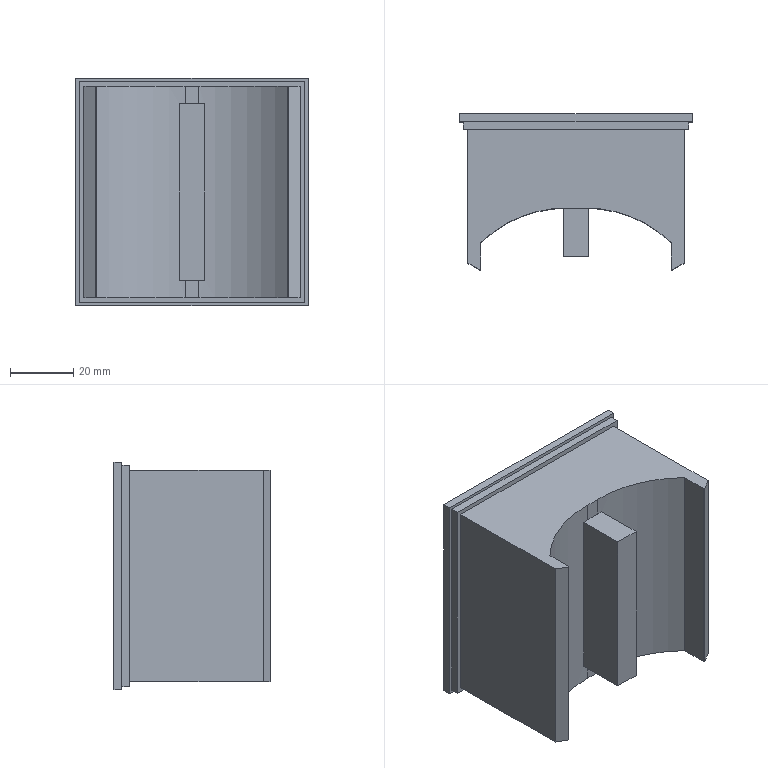Part | SolidWorks | features ICE 4, Extrusion 1 | 1 solid | 36 faces | box 73.144 x 49.228 x 71.78 mm | volume 167014 mm3 | plane 28 | cylinder 8 | commonest cylinder face diameters 3 x4 0.46 x2 77.24 x2
STEP:
#1=CARTESIAN_POINT('',(1.5,16.101,-56.78));
#2=VERTEX_POINT('',#1);
#3=CARTESIAN_POINT('',(-1.5,16.101,-56.78));
#4=VERTEX_POINT('',#3);
#5=CARTESIAN_POINT('',(0.,16.101,-56.78));
#6=DIRECTION('',(0.,0.,-1.));
#7=DIRECTION('',(-1.,0.,0.));
#8=AXIS2_PLACEMENT_3D('',#5,#6,#7);
#9=CIRCLE('',#8,1.5);
#10=EDGE_CURVE('',#2,#4,#9,.T.);
#11=ORIENTED_EDGE('',*,*,#10,.F.);
#12=CARTESIAN_POINT('',(1.5,16.101,-66.78));
#13=VERTEX_POINT('',#12);
#14=CARTESIAN_POINT('',(1.5,16.101,-56.78));
#15=DIRECTION('',(0.,0.,-1.));
#16=VECTOR('',#15,1000.);
#17=LINE('',#14,#16);
#18=EDGE_CURVE('',#2,#13,#17,.T.);
#19=ORIENTED_EDGE('',*,*,#18,.T.);
#20=CARTESIAN_POINT('',(-1.5,16.101,-66.78));
#21=VERTEX_POINT('',#20);
#22=CARTESIAN_POINT('',(0.,16.101,-66.78));
#23=DIRECTION('',(0.,0.,-1.));
#24=DIRECTION('',(-1.,0.,0.));
#25=AXIS2_PLACEMENT_3D('',#22,#23,#24);
#26=CIRCLE('',#25,1.5);
#27=EDGE_CURVE('',#13,#21,#26,.T.);
#28=ORIENTED_EDGE('',*,*,#27,.T.);
#29=CARTESIAN_POINT('',(-1.5,16.101,-56.78));
#30=DIRECTION('',(0.,0.,-1.));
#31=VECTOR('',#30,1000.);
#32=LINE('',#29,#31);
#33=EDGE_CURVE('',#4,#21,#32,.T.);
#34=ORIENTED_EDGE('',*,*,#33,.F.);
#35=EDGE_LOOP('',(#11,#19,#28,#34));
#36=FACE_OUTER_BOUND('',#35,.T.);
#37=CARTESIAN_POINT('',(0.,16.101,-56.78));
#38=DIRECTION('',(0.,0.,-1.));
#39=DIRECTION('',(-1.,0.,0.));
#40=AXIS2_PLACEMENT_3D('',#37,#38,#39);
#41=CYLINDRICAL_SURFACE('',#40,1.5);
#42=ADVANCED_FACE('',(#36),#41,.F.);
#43=CARTESIAN_POINT('',(1.5,6.101,-56.78));
#44=VERTEX_POINT('',#43);
#45=CARTESIAN_POINT('',(-1.5,6.101,-56.78));
#46=VERTEX_POINT('',#45);
#47=CARTESIAN_POINT('',(0.,6.101,-56.78));
#48=DIRECTION('',(0.,0.,-1.));
#49=DIRECTION('',(-1.,0.,0.));
#50=AXIS2_PLACEMENT_3D('',#47,#48,#49);
#51=CIRCLE('',#50,1.5);
#52=EDGE_CURVE('',#44,#46,#51,.T.);
#53=ORIENTED_EDGE('',*,*,#52,.F.);
#54=CARTESIAN_POINT('',(1.5,6.101,-66.78));
#55=VERTEX_POINT('',#54);
#56=CARTESIAN_POINT('',(1.5,6.101,-56.78));
#57=DIRECTION('',(0.,0.,-1.));
#58=VECTOR('',#57,1000.);
#59=LINE('',#56,#58);
#60=EDGE_CURVE('',#44,#55,#59,.T.);
#61=ORIENTED_EDGE('',*,*,#60,.T.);
#62=CARTESIAN_POINT('',(-1.5,6.101,-66.78));
#63=VERTEX_POINT('',#62);
#64=CARTESIAN_POINT('',(0.,6.101,-66.78));
#65=DIRECTION('',(0.,0.,-1.));
#66=DIRECTION('',(-1.,0.,0.));
#67=AXIS2_PLACEMENT_3D('',#64,#65,#66);
#68=CIRCLE('',#67,1.5);
#69=EDGE_CURVE('',#55,#63,#68,.T.);
#70=ORIENTED_EDGE('',*,*,#69,.T.);
#71=CARTESIAN_POINT('',(-1.5,6.101,-56.78));
#72=DIRECTION('',(0.,0.,-1.));
#73=VECTOR('',#72,1000.);
#74=LINE('',#71,#73);
#75=EDGE_CURVE('',#46,#63,#74,.T.);
#76=ORIENTED_EDGE('',*,*,#75,.F.);
#77=EDGE_LOOP('',(#53,#61,#70,#76));
#78=FACE_OUTER_BOUND('',#77,.T.);
#79=CARTESIAN_POINT('',(0.,6.101,-56.78));
#80=DIRECTION('',(0.,0.,-1.));
#81=DIRECTION('',(-1.,0.,0.));
#82=AXIS2_PLACEMENT_3D('',#79,#80,#81);
#83=CYLINDRICAL_SURFACE('',#82,1.5);
#84=ADVANCED_FACE('',(#78),#83,.F.);
#85=CARTESIAN_POINT('',(-2.201,0.77,-61.17));
#86=VERTEX_POINT('',#85);
#87=CARTESIAN_POINT('',(2.201,0.77,-61.17));
#88=VERTEX_POINT('',#87);
#89=CARTESIAN_POINT('',(0.,0.77,-61.17));
#90=DIRECTION('',(1.,0.,0.));
#91=VECTOR('',#90,1000.);
#92=LINE('',#89,#91);
#93=EDGE_CURVE('',#86,#88,#92,.T.);
#94=ORIENTED_EDGE('',*,*,#93,.F.);
#95=CARTESIAN_POINT('',(-2.201,0.77,-66.78));
#96=VERTEX_POINT('',#95);
#97=CARTESIAN_POINT('',(-2.201,0.77,-66.78));
#98=DIRECTION('',(0.,0.,1.));
#99=VECTOR('',#98,1000.);
#100=LINE('',#97,#99);
#101=EDGE_CURVE('',#96,#86,#100,.T.);
#102=ORIENTED_EDGE('',*,*,#101,.F.);
#103=CARTESIAN_POINT('',(2.201,0.77,-66.78));
#104=VERTEX_POINT('',#103);
#105=CARTESIAN_POINT('',(0.,0.77,-66.78));
#106=DIRECTION('',(1.,0.,0.));
#107=VECTOR('',#106,1000.);
#108=LINE('',#105,#107);
#109=EDGE_CURVE('',#96,#104,#108,.T.);
#110=ORIENTED_EDGE('',*,*,#109,.T.);
#111=CARTESIAN_POINT('',(2.201,0.77,-66.78));
#112=DIRECTION('',(0.,0.,1.));
#113=VECTOR('',#112,1000.);
#114=LINE('',#111,#113);
#115=EDGE_CURVE('',#104,#88,#114,.T.);
#116=ORIENTED_EDGE('',*,*,#115,.T.);
#117=EDGE_LOOP('',(#94,#102,#110,#116));
#118=FACE_OUTER_BOUND('',#117,.T.);
#119=CARTESIAN_POINT('',(0.,0.77,-66.78));
#120=DIRECTION('',(0.,-1.,0.));
#121=DIRECTION('',(1.,0.,0.));
#122=AXIS2_PLACEMENT_3D('',#119,#120,#121);
#123=PLANE('',#122);
#124=ADVANCED_FACE('',(#118),#123,.T.);
#125=CARTESIAN_POINT('',(-34.072,25.498,0.));
#126=VERTEX_POINT('',#125);
#127=CARTESIAN_POINT('',(-34.072,-16.562,0.));
#128=VERTEX_POINT('',#127);
#129=CARTESIAN_POINT('',(-34.072,-16.562,0.));
#130=DIRECTION('',(0.,-1.,0.));
#131=VECTOR('',#130,1000.);
#132=LINE('',#129,#131);
#133=EDGE_CURVE('',#126,#128,#132,.T.);
#134=ORIENTED_EDGE('',*,*,#133,.F.);
#135=CARTESIAN_POINT('',(-34.072,25.498,-66.78));
#136=VERTEX_POINT('',#135);
#137=CARTESIAN_POINT('',(-34.072,25.498,-66.78));
#138=DIRECTION('',(0.,0.,1.));
#139=VECTOR('',#138,1000.);
#140=LINE('',#137,#139);
#141=EDGE_CURVE('',#136,#126,#140,.T.);
#142=ORIENTED_EDGE('',*,*,#141,.F.);
#143=CARTESIAN_POINT('',(-34.072,-16.562,-66.78));
#144=VERTEX_POINT('',#143);
#145=CARTESIAN_POINT('',(-34.072,-16.562,-66.78));
#146=DIRECTION('',(0.,-1.,0.));
#147=VECTOR('',#146,1000.);
#148=LINE('',#145,#147);
#149=EDGE_CURVE('',#136,#144,#148,.T.);
#150=ORIENTED_EDGE('',*,*,#149,.T.);
#151=CARTESIAN_POINT('',(-34.072,-16.562,-66.78));
#152=DIRECTION('',(0.,0.,1.));
#153=VECTOR('',#152,1000.);
#154=LINE('',#151,#153);
#155=EDGE_CURVE('',#144,#128,#154,.T.);
#156=ORIENTED_EDGE('',*,*,#155,.T.);
#157=EDGE_LOOP('',(#134,#142,#150,#156));
#158=FACE_OUTER_BOUND('',#157,.T.);
#159=CARTESIAN_POINT('',(-34.072,-16.562,-66.78));
#160=DIRECTION('',(-1.,0.,0.));
#161=DIRECTION('',(0.,0.,1.));
#162=AXIS2_PLACEMENT_3D('',#159,#160,#161);
#163=PLANE('',#162);
#164=ADVANCED_FACE('',(#158),#163,.T.);
#165=CARTESIAN_POINT('',(34.072,-16.562,0.));
#166=VERTEX_POINT('',#165);
#167=CARTESIAN_POINT('',(34.072,25.498,0.));
#168=VERTEX_POINT('',#167);
#169=CARTESIAN_POINT('',(34.072,-16.562,0.));
#170=DIRECTION('',(0.,1.,0.));
#171=VECTOR('',#170,1000.);
#172=LINE('',#169,#171);
#173=EDGE_CURVE('',#166,#168,#172,.T.);
#174=ORIENTED_EDGE('',*,*,#173,.F.);
#175=CARTESIAN_POINT('',(34.072,-16.562,-66.78));
#176=VERTEX_POINT('',#175);
#177=CARTESIAN_POINT('',(34.072,-16.562,-66.78));
#178=DIRECTION('',(0.,0.,1.));
#179=VECTOR('',#178,1000.);
#180=LINE('',#177,#179);
#181=EDGE_CURVE('',#176,#166,#180,.T.);
#182=ORIENTED_EDGE('',*,*,#181,.F.);
#183=CARTESIAN_POINT('',(34.072,25.498,-66.78));
#184=VERTEX_POINT('',#183);
#185=CARTESIAN_POINT('',(34.072,-16.562,-66.78));
#186=DIRECTION('',(0.,1.,0.));
#187=VECTOR('',#186,1000.);
#188=LINE('',#185,#187);
#189=EDGE_CURVE('',#176,#184,#188,.T.);
#190=ORIENTED_EDGE('',*,*,#189,.T.);
#191=CARTESIAN_POINT('',(34.072,25.498,-66.78));
#192=DIRECTION('',(0.,0.,1.));
#193=VECTOR('',#192,1000.);
#194=LINE('',#191,#193);
#195=EDGE_CURVE('',#184,#168,#194,.T.);
#196=ORIENTED_EDGE('',*,*,#195,.T.);
#197=EDGE_LOOP('',(#174,#182,#190,#196));
#198=FACE_OUTER_BOUND('',#197,.T.);
#199=CARTESIAN_POINT('',(34.072,-16.562,-66.78));
#200=DIRECTION('',(1.,0.,0.));
#201=DIRECTION('',(0.,1.,0.));
#202=AXIS2_PLACEMENT_3D('',#199,#200,#201);
#203=PLANE('',#202);
#204=ADVANCED_FACE('',(#198),#203,.T.);
#205=CARTESIAN_POINT('',(30.37,-18.699,0.));
#206=VERTEX_POINT('',#205);
#207=CARTESIAN_POINT('',(30.37,-18.699,0.));
#208=DIRECTION('',(0.866,0.5,0.));
#209=VECTOR('',#208,1000.);
#210=LINE('',#207,#209);
#211=EDGE_CURVE('',#206,#166,#210,.T.);
#212=ORIENTED_EDGE('',*,*,#211,.F.);
#213=CARTESIAN_POINT('',(30.37,-18.699,-66.78));
#214=VERTEX_POINT('',#213);
#215=CARTESIAN_POINT('',(30.37,-18.699,-66.78));
#216=DIRECTION('',(0.,0.,1.));
#217=VECTOR('',#216,1000.);
#218=LINE('',#215,#217);
#219=EDGE_CURVE('',#214,#206,#218,.T.);
#220=ORIENTED_EDGE('',*,*,#219,.F.);
#221=CARTESIAN_POINT('',(30.37,-18.699,-66.78));
#222=DIRECTION('',(0.866,0.5,0.));
#223=VECTOR('',#222,1000.);
#224=LINE('',#221,#223);
#225=EDGE_CURVE('',#214,#176,#224,.T.);
#226=ORIENTED_EDGE('',*,*,#225,.T.);
#227=ORIENTED_EDGE('',*,*,#181,.T.);
#228=EDGE_LOOP('',(#212,#220,#226,#227));
#229=FACE_OUTER_BOUND('',#228,.T.);
#230=CARTESIAN_POINT('',(30.37,-18.699,-66.78));
#231=DIRECTION('',(0.5,-0.866,0.));
#232=DIRECTION('',(0.866,0.5,0.));
#233=AXIS2_PLACEMENT_3D('',#230,#231,#232);
#234=PLANE('',#233);
#235=ADVANCED_FACE('',(#229),#234,.T.);
#236=CARTESIAN_POINT('',(30.025,-18.5,0.));
#237=VERTEX_POINT('',#236);
#238=CARTESIAN_POINT('',(30.255,-18.5,0.));
#239=DIRECTION('',(0.,0.,1.));
#240=DIRECTION('',(-1.,0.,0.));
#241=AXIS2_PLACEMENT_3D('',#238,#239,#240);
#242=CIRCLE('',#241,0.23);
#243=EDGE_CURVE('',#237,#206,#242,.T.);
#244=ORIENTED_EDGE('',*,*,#243,.F.);
#245=CARTESIAN_POINT('',(30.025,-18.5,-66.78));
#246=VERTEX_POINT('',#245);
#247=CARTESIAN_POINT('',(30.025,-18.5,-66.78));
#248=DIRECTION('',(0.,0.,1.));
#249=VECTOR('',#248,1000.);
#250=LINE('',#247,#249);
#251=EDGE_CURVE('',#246,#237,#250,.T.);
#252=ORIENTED_EDGE('',*,*,#251,.F.);
#253=CARTESIAN_POINT('',(30.255,-18.5,-66.78));
#254=DIRECTION('',(0.,0.,1.));
#255=DIRECTION('',(-1.,0.,0.));
#256=AXIS2_PLACEMENT_3D('',#253,#254,#255);
#257=CIRCLE('',#256,0.23);
#258=EDGE_CURVE('',#246,#214,#257,.T.);
#259=ORIENTED_EDGE('',*,*,#258,.T.);
#260=ORIENTED_EDGE('',*,*,#219,.T.);
#261=EDGE_LOOP('',(#244,#252,#259,#260));
#262=FACE_OUTER_BOUND('',#261,.T.);
#263=CARTESIAN_POINT('',(30.255,-18.5,-66.78));
#264=DIRECTION('',(0.,0.,1.));
#265=DIRECTION('',(1.,0.,0.));
#266=AXIS2_PLACEMENT_3D('',#263,#264,#265);
#267=CYLINDRICAL_SURFACE('',#266,0.23);
#268=ADVANCED_FACE('',(#262),#267,.T.);
#269=CARTESIAN_POINT('',(30.025,-10.173,0.));
#270=VERTEX_POINT('',#269);
#271=CARTESIAN_POINT('',(30.025,-10.173,0.));
#272=DIRECTION('',(0.,-1.,0.));
#273=VECTOR('',#272,1000.);
#274=LINE('',#271,#273);
#275=EDGE_CURVE('',#270,#237,#274,.T.);
#276=ORIENTED_EDGE('',*,*,#275,.F.);
#277=CARTESIAN_POINT('',(30.025,-10.173,-66.78));
#278=VERTEX_POINT('',#277);
#279=CARTESIAN_POINT('',(30.025,-10.173,-66.78));
#280=DIRECTION('',(0.,0.,1.));
#281=VECTOR('',#280,1000.);
#282=LINE('',#279,#281);
#283=EDGE_CURVE('',#278,#270,#282,.T.);
#284=ORIENTED_EDGE('',*,*,#283,.F.);
#285=CARTESIAN_POINT('',(30.025,-10.173,-66.78));
#286=DIRECTION('',(0.,-1.,0.));
#287=VECTOR('',#286,1000.);
#288=LINE('',#285,#287);
#289=EDGE_CURVE('',#278,#246,#288,.T.);
#290=ORIENTED_EDGE('',*,*,#289,.T.);
#291=ORIENTED_EDGE('',*,*,#251,.T.);
#292=EDGE_LOOP('',(#276,#284,#290,#291));
#293=FACE_OUTER_BOUND('',#292,.T.);
#294=CARTESIAN_POINT('',(30.025,-10.173,-66.78));
#295=DIRECTION('',(-1.,0.,0.));
#296=DIRECTION('',(0.,-1.,0.));
#297=AXIS2_PLACEMENT_3D('',#294,#295,#296);
#298=PLANE('',#297);
#299=ADVANCED_FACE('',(#293),#298,.T.);
#300=CARTESIAN_POINT('',(4.03,0.7683,-61.17));
#301=VERTEX_POINT('',#300);
#302=CARTESIAN_POINT('',(3.08,-37.84,-61.17));
#303=DIRECTION('',(0.,0.,-1.));
#304=DIRECTION('',(-1.,0.,0.));
#305=AXIS2_PLACEMENT_3D('',#302,#303,#304);
#306=CIRCLE('',#305,38.62);
#307=EDGE_CURVE('',#88,#301,#306,.T.);
#308=ORIENTED_EDGE('',*,*,#307,.F.);
#309=ORIENTED_EDGE('',*,*,#115,.F.);
#310=CARTESIAN_POINT('',(3.08,-37.84,-66.78));
#311=DIRECTION('',(0.,0.,-1.));
#312=DIRECTION('',(-1.,0.,0.));
#313=AXIS2_PLACEMENT_3D('',#310,#311,#312);
#314=CIRCLE('',#313,38.62);
#315=EDGE_CURVE('',#104,#278,#314,.T.);
#316=ORIENTED_EDGE('',*,*,#315,.T.);
#317=ORIENTED_EDGE('',*,*,#283,.T.);
#318=CARTESIAN_POINT('',(2.201,0.77,0.));
#319=VERTEX_POINT('',#318);
#320=CARTESIAN_POINT('',(3.08,-37.84,0.));
#321=DIRECTION('',(0.,0.,-1.));
#322=DIRECTION('',(-1.,0.,0.));
#323=AXIS2_PLACEMENT_3D('',#320,#321,#322);
#324=CIRCLE('',#323,38.62);
#325=EDGE_CURVE('',#319,#270,#324,.T.);
#326=ORIENTED_EDGE('',*,*,#325,.F.);
#327=CARTESIAN_POINT('',(2.201,0.77,-5.61));
#328=VERTEX_POINT('',#327);
#329=CARTESIAN_POINT('',(2.201,0.77,-66.78));
#330=DIRECTION('',(0.,0.,1.));
#331=VECTOR('',#330,1000.);
#332=LINE('',#329,#331);
#333=EDGE_CURVE('',#328,#319,#332,.T.);
#334=ORIENTED_EDGE('',*,*,#333,.F.);
#335=CARTESIAN_POINT('',(4.03,0.7683,-5.61));
#336=VERTEX_POINT('',#335);
#337=CARTESIAN_POINT('',(3.08,-37.84,-5.61));
#338=DIRECTION('',(0.,0.,1.));
#339=DIRECTION('',(1.,0.,0.));
#340=AXIS2_PLACEMENT_3D('',#337,#338,#339);
#341=CIRCLE('',#340,38.62);
#342=EDGE_CURVE('',#336,#328,#341,.T.);
#343=ORIENTED_EDGE('',*,*,#342,.F.);
#344=CARTESIAN_POINT('',(4.03,0.7683,-66.78));
#345=DIRECTION('',(0.,0.,1.));
#346=VECTOR('',#345,1000.);
#347=LINE('',#344,#346);
#348=EDGE_CURVE('',#301,#336,#347,.T.);
#349=ORIENTED_EDGE('',*,*,#348,.F.);
#350=EDGE_LOOP('',(#308,#309,#316,#317,#326,#334,#343,#349));
#351=FACE_OUTER_BOUND('',#350,.T.);
#352=CARTESIAN_POINT('',(3.08,-37.84,-66.78));
#353=DIRECTION('',(0.,0.,1.));
#354=DIRECTION('',(1.,0.,0.));
#355=AXIS2_PLACEMENT_3D('',#352,#353,#354);
#356=CYLINDRICAL_SURFACE('',#355,38.62);
#357=ADVANCED_FACE('',(#351),#356,.F.);
#358=CARTESIAN_POINT('',(-2.201,0.77,-5.61));
#359=VERTEX_POINT('',#358);
#360=CARTESIAN_POINT('',(0.,0.77,-5.61));
#361=DIRECTION('',(-1.,0.,0.));
#362=VECTOR('',#361,1000.);
#363=LINE('',#360,#362);
#364=EDGE_CURVE('',#328,#359,#363,.T.);
#365=ORIENTED_EDGE('',*,*,#364,.F.);
#366=ORIENTED_EDGE('',*,*,#333,.T.);
#367=CARTESIAN_POINT('',(-2.201,0.77,0.));
#368=VERTEX_POINT('',#367);
#369=CARTESIAN_POINT('',(0.,0.77,0.));
#370=DIRECTION('',(1.,0.,0.));
#371=VECTOR('',#370,1000.);
#372=LINE('',#369,#371);
#373=EDGE_CURVE('',#368,#319,#372,.T.);
#374=ORIENTED_EDGE('',*,*,#373,.F.);
#375=CARTESIAN_POINT('',(-2.201,0.77,-66.78));
#376=DIRECTION('',(0.,0.,1.));
#377=VECTOR('',#376,1000.);
#378=LINE('',#375,#377);
#379=EDGE_CURVE('',#359,#368,#378,.T.);
#380=ORIENTED_EDGE('',*,*,#379,.F.);
#381=EDGE_LOOP('',(#365,#366,#374,#380));
#382=FACE_OUTER_BOUND('',#381,.T.);
#383=CARTESIAN_POINT('',(0.,0.77,-66.78));
#384=DIRECTION('',(0.,-1.,0.));
#385=DIRECTION('',(1.,0.,0.));
#386=AXIS2_PLACEMENT_3D('',#383,#384,#385);
#387=PLANE('',#386);
#388=ADVANCED_FACE('',(#382),#387,.T.);
#389=CARTESIAN_POINT('',(-4.03,0.7683,-61.17));
#390=VERTEX_POINT('',#389);
#391=CARTESIAN_POINT('',(-3.08,-37.84,-61.17));
#392=DIRECTION('',(0.,0.,-1.));
#393=DIRECTION('',(-1.,0.,0.));
#394=AXIS2_PLACEMENT_3D('',#391,#392,#393);
#395=CIRCLE('',#394,38.62);
#396=EDGE_CURVE('',#390,#86,#395,.T.);
#397=ORIENTED_EDGE('',*,*,#396,.F.);
#398=CARTESIAN_POINT('',(-4.03,0.7683,-5.61));
#399=VERTEX_POINT('',#398);
#400=CARTESIAN_POINT('',(-4.03,0.7683,-66.78));
#401=DIRECTION('',(0.,0.,-1.));
#402=VECTOR('',#401,1000.);
#403=LINE('',#400,#402);
#404=EDGE_CURVE('',#399,#390,#403,.T.);
#405=ORIENTED_EDGE('',*,*,#404,.F.);
#406=CARTESIAN_POINT('',(-3.08,-37.84,-5.61));
#407=DIRECTION('',(0.,0.,1.));
#408=DIRECTION('',(1.,0.,0.));
#409=AXIS2_PLACEMENT_3D('',#406,#407,#408);
#410=CIRCLE('',#409,38.62);
#411=EDGE_CURVE('',#359,#399,#410,.T.);
#412=ORIENTED_EDGE('',*,*,#411,.F.);
#413=ORIENTED_EDGE('',*,*,#379,.T.);
#414=CARTESIAN_POINT('',(-30.025,-10.173,0.));
#415=VERTEX_POINT('',#414);
#416=CARTESIAN_POINT('',(-3.08,-37.84,0.));
#417=DIRECTION('',(0.,0.,-1.));
#418=DIRECTION('',(1.,0.,0.));
#419=AXIS2_PLACEMENT_3D('',#416,#417,#418);
#420=CIRCLE('',#419,38.62);
#421=EDGE_CURVE('',#415,#368,#420,.T.);
#422=ORIENTED_EDGE('',*,*,#421,.F.);
#423=CARTESIAN_POINT('',(-30.025,-10.173,-66.78));
#424=VERTEX_POINT('',#423);
#425=CARTESIAN_POINT('',(-30.025,-10.173,-66.78));
#426=DIRECTION('',(0.,0.,1.));
#427=VECTOR('',#426,1000.);
#428=LINE('',#425,#427);
#429=EDGE_CURVE('',#424,#415,#428,.T.);
#430=ORIENTED_EDGE('',*,*,#429,.F.);
#431=CARTESIAN_POINT('',(-3.08,-37.84,-66.78));
#432=DIRECTION('',(0.,0.,-1.));
#433=DIRECTION('',(1.,0.,0.));
#434=AXIS2_PLACEMENT_3D('',#431,#432,#433);
#435=CIRCLE('',#434,38.62);
#436=EDGE_CURVE('',#424,#96,#435,.T.);
#437=ORIENTED_EDGE('',*,*,#436,.T.);
#438=ORIENTED_EDGE('',*,*,#101,.T.);
#439=EDGE_LOOP('',(#397,#405,#412,#413,#422,#430,#437,#438));
#440=FACE_OUTER_BOUND('',#439,.T.);
#441=CARTESIAN_POINT('',(-3.08,-37.84,-66.78));
#442=DIRECTION('',(0.,0.,1.));
#443=DIRECTION('',(1.,0.,0.));
#444=AXIS2_PLACEMENT_3D('',#441,#442,#443);
#445=CYLINDRICAL_SURFACE('',#444,38.62);
#446=ADVANCED_FACE('',(#440),#445,.F.);
#447=CARTESIAN_POINT('',(-30.025,-18.5,0.));
#448=VERTEX_POINT('',#447);
#449=CARTESIAN_POINT('',(-30.025,-10.173,0.));
#450=DIRECTION('',(0.,1.,0.));
#451=VECTOR('',#450,1000.);
#452=LINE('',#449,#451);
#453=EDGE_CURVE('',#448,#415,#452,.T.);
#454=ORIENTED_EDGE('',*,*,#453,.F.);
#455=CARTESIAN_POINT('',(-30.025,-18.5,-66.78));
#456=VERTEX_POINT('',#455);
#457=CARTESIAN_POINT('',(-30.025,-18.5,-66.78));
#458=DIRECTION('',(0.,0.,1.));
#459=VECTOR('',#458,1000.);
#460=LINE('',#457,#459);
#461=EDGE_CURVE('',#456,#448,#460,.T.);
#462=ORIENTED_EDGE('',*,*,#461,.F.);
#463=CARTESIAN_POINT('',(-30.025,-10.173,-66.78));
#464=DIRECTION('',(0.,1.,0.));
#465=VECTOR('',#464,1000.);
#466=LINE('',#463,#465);
#467=EDGE_CURVE('',#456,#424,#466,.T.);
#468=ORIENTED_EDGE('',*,*,#467,.T.);
#469=ORIENTED_EDGE('',*,*,#429,.T.);
#470=EDGE_LOOP('',(#454,#462,#468,#469));
#471=FACE_OUTER_BOUND('',#470,.T.);
#472=CARTESIAN_POINT('',(-30.025,-10.173,-66.78));
#473=DIRECTION('',(1.,0.,0.));
#474=DIRECTION('',(0.,1.,0.));
#475=AXIS2_PLACEMENT_3D('',#472,#473,#474);
#476=PLANE('',#475);
#477=ADVANCED_FACE('',(#471),#476,.T.);
#478=CARTESIAN_POINT('',(-30.37,-18.699,0.));
#479=VERTEX_POINT('',#478);
#480=CARTESIAN_POINT('',(-30.255,-18.5,0.));
#481=DIRECTION('',(0.,0.,1.));
#482=DIRECTION('',(1.,0.,0.));
#483=AXIS2_PLACEMENT_3D('',#480,#481,#482);
#484=CIRCLE('',#483,0.23);
#485=EDGE_CURVE('',#479,#448,#484,.T.);
#486=ORIENTED_EDGE('',*,*,#485,.F.);
#487=CARTESIAN_POINT('',(-30.37,-18.699,-66.78));
#488=VERTEX_POINT('',#487);
#489=CARTESIAN_POINT('',(-30.37,-18.699,-66.78));
#490=DIRECTION('',(0.,0.,1.));
#491=VECTOR('',#490,1000.);
#492=LINE('',#489,#491);
#493=EDGE_CURVE('',#488,#479,#492,.T.);
#494=ORIENTED_EDGE('',*,*,#493,.F.);
#495=CARTESIAN_POINT('',(-30.255,-18.5,-66.78));
#496=DIRECTION('',(0.,0.,1.));
#497=DIRECTION('',(1.,0.,0.));
#498=AXIS2_PLACEMENT_3D('',#495,#496,#497);
#499=CIRCLE('',#498,0.23);
#500=EDGE_CURVE('',#488,#456,#499,.T.);
#501=ORIENTED_EDGE('',*,*,#500,.T.);
#502=ORIENTED_EDGE('',*,*,#461,.T.);
#503=EDGE_LOOP('',(#486,#494,#501,#502));
#504=FACE_OUTER_BOUND('',#503,.T.);
#505=CARTESIAN_POINT('',(-30.255,-18.5,-66.78));
#506=DIRECTION('',(0.,0.,1.));
#507=DIRECTION('',(1.,0.,0.));
#508=AXIS2_PLACEMENT_3D('',#505,#506,#507);
#509=CYLINDRICAL_SURFACE('',#508,0.23);
#510=ADVANCED_FACE('',(#504),#509,.T.);
#511=CARTESIAN_POINT('',(-30.37,-18.699,0.));
#512=DIRECTION('',(0.866,-0.5,0.));
#513=VECTOR('',#512,1000.);
#514=LINE('',#511,#513);
#515=EDGE_CURVE('',#128,#479,#514,.T.);
#516=ORIENTED_EDGE('',*,*,#515,.F.);
#517=ORIENTED_EDGE('',*,*,#155,.F.);
#518=CARTESIAN_POINT('',(-30.37,-18.699,-66.78));
#519=DIRECTION('',(0.866,-0.5,0.));
#520=VECTOR('',#519,1000.);
#521=LINE('',#518,#520);
#522=EDGE_CURVE('',#144,#488,#521,.T.);
#523=ORIENTED_EDGE('',*,*,#522,.T.);
#524=ORIENTED_EDGE('',*,*,#493,.T.);
#525=EDGE_LOOP('',(#516,#517,#523,#524));
#526=FACE_OUTER_BOUND('',#525,.T.);
#527=CARTESIAN_POINT('',(-30.37,-18.699,-66.78));
#528=DIRECTION('',(-0.5,-0.866,0.));
#529=DIRECTION('',(0.866,-0.5,0.));
#530=AXIS2_PLACEMENT_3D('',#527,#528,#529);
#531=PLANE('',#530);
#532=ADVANCED_FACE('',(#526),#531,.T.);
#533=CARTESIAN_POINT('',(0.,16.101,-66.78));
#534=DIRECTION('',(0.,0.,-1.));
#535=DIRECTION('',(-1.,0.,0.));
#536=AXIS2_PLACEMENT_3D('',#533,#534,#535);
#537=CIRCLE('',#536,1.5);
#538=EDGE_CURVE('',#21,#13,#537,.T.);
#539=ORIENTED_EDGE('',*,*,#538,.F.);
#540=ORIENTED_EDGE('',*,*,#27,.F.);
#541=EDGE_LOOP('',(#539,#540));
#542=FACE_BOUND('',#541,.T.);
#543=CARTESIAN_POINT('',(0.,6.101,-66.78));
#544=DIRECTION('',(0.,0.,-1.));
#545=DIRECTION('',(-1.,0.,0.));
#546=AXIS2_PLACEMENT_3D('',#543,#544,#545);
#547=CIRCLE('',#546,1.5);
#548=EDGE_CURVE('',#63,#55,#547,.T.);
#549=ORIENTED_EDGE('',*,*,#548,.F.);
#550=ORIENTED_EDGE('',*,*,#69,.F.);
#551=EDGE_LOOP('',(#549,#550));
#552=FACE_BOUND('',#551,.T.);
#553=ORIENTED_EDGE('',*,*,#149,.F.);
#554=CARTESIAN_POINT('',(-34.072,25.498,-66.78));
#555=DIRECTION('',(-1.,0.,0.));
#556=VECTOR('',#555,1000.);
#557=LINE('',#554,#556);
#558=EDGE_CURVE('',#184,#136,#557,.T.);
#559=ORIENTED_EDGE('',*,*,#558,.F.);
#560=ORIENTED_EDGE('',*,*,#189,.F.);
#561=ORIENTED_EDGE('',*,*,#225,.F.);
#562=ORIENTED_EDGE('',*,*,#258,.F.);
#563=ORIENTED_EDGE('',*,*,#289,.F.);
#564=ORIENTED_EDGE('',*,*,#315,.F.);
#565=ORIENTED_EDGE('',*,*,#109,.F.);
#566=ORIENTED_EDGE('',*,*,#436,.F.);
#567=ORIENTED_EDGE('',*,*,#467,.F.);
#568=ORIENTED_EDGE('',*,*,#500,.F.);
#569=ORIENTED_EDGE('',*,*,#522,.F.);
#570=EDGE_LOOP('',(#553,#559,#560,#561,#562,#563,#564,#565,#566,#567,#568,#569));
#571=FACE_OUTER_BOUND('',#570,.T.);
#572=CARTESIAN_POINT('',(30.255,-18.5,-66.78));
#573=DIRECTION('',(0.,0.,-1.));
#574=DIRECTION('',(-1.,0.,0.));
#575=AXIS2_PLACEMENT_3D('',#572,#573,#574);
#576=PLANE('',#575);
#577=ADVANCED_FACE('',(#542,#552,#571),#576,.T.);
#578=ORIENTED_EDGE('',*,*,#133,.T.);
#579=ORIENTED_EDGE('',*,*,#515,.T.);
#580=ORIENTED_EDGE('',*,*,#485,.T.);
#581=ORIENTED_EDGE('',*,*,#453,.T.);
#582=ORIENTED_EDGE('',*,*,#421,.T.);
#583=ORIENTED_EDGE('',*,*,#373,.T.);
#584=ORIENTED_EDGE('',*,*,#325,.T.);
#585=ORIENTED_EDGE('',*,*,#275,.T.);
#586=ORIENTED_EDGE('',*,*,#243,.T.);
#587=ORIENTED_EDGE('',*,*,#211,.T.);
#588=ORIENTED_EDGE('',*,*,#173,.T.);
#589=CARTESIAN_POINT('',(-34.072,25.498,0.));
#590=DIRECTION('',(-1.,0.,0.));
#591=VECTOR('',#590,1000.);
#592=LINE('',#589,#591);
#593=EDGE_CURVE('',#168,#126,#592,.T.);
#594=ORIENTED_EDGE('',*,*,#593,.T.);
#595=EDGE_LOOP('',(#578,#579,#580,#581,#582,#583,#584,#585,#586,#587,#588,#594));
#596=FACE_OUTER_BOUND('',#595,.T.);
#597=CARTESIAN_POINT('',(30.255,-18.5,0.));
#598=DIRECTION('',(0.,0.,-1.));
#599=DIRECTION('',(-1.,0.,0.));
#600=AXIS2_PLACEMENT_3D('',#597,#598,#599);
#601=PLANE('',#600);
#602=ADVANCED_FACE('',(#596),#601,.F.);
#603=ORIENTED_EDGE('',*,*,#93,.T.);
#604=ORIENTED_EDGE('',*,*,#307,.T.);
#605=CARTESIAN_POINT('',(4.03,-14.502,-61.17));
#606=VERTEX_POINT('',#605);
#607=CARTESIAN_POINT('',(4.03,-14.502,-61.17));
#608=DIRECTION('',(0.,1.,0.));
#609=VECTOR('',#608,1000.);
#610=LINE('',#607,#609);
#611=EDGE_CURVE('',#606,#301,#610,.T.);
#612=ORIENTED_EDGE('',*,*,#611,.F.);
#613=CARTESIAN_POINT('',(-4.03,-14.502,-61.17));
#614=VERTEX_POINT('',#613);
#615=CARTESIAN_POINT('',(4.03,-14.502,-61.17));
#616=DIRECTION('',(-1.,0.,0.));
#617=VECTOR('',#616,1000.);
#618=LINE('',#615,#617);
#619=EDGE_CURVE('',#606,#614,#618,.T.);
#620=ORIENTED_EDGE('',*,*,#619,.T.);
#621=CARTESIAN_POINT('',(-4.03,-14.502,-61.17));
#622=DIRECTION('',(0.,1.,0.));
#623=VECTOR('',#622,1000.);
#624=LINE('',#621,#623);
#625=EDGE_CURVE('',#614,#390,#624,.T.);
#626=ORIENTED_EDGE('',*,*,#625,.T.);
#627=ORIENTED_EDGE('',*,*,#396,.T.);
#628=EDGE_LOOP('',(#603,#604,#612,#620,#626,#627));
#629=FACE_OUTER_BOUND('',#628,.T.);
#630=CARTESIAN_POINT('',(4.03,-14.502,-61.17));
#631=DIRECTION('',(0.,0.,-1.));
#632=DIRECTION('',(-1.,0.,0.));
#633=AXIS2_PLACEMENT_3D('',#630,#631,#632);
#634=PLANE('',#633);
#635=ADVANCED_FACE('',(#629),#634,.T.);
#636=ORIENTED_EDGE('',*,*,#611,.T.);
#637=ORIENTED_EDGE('',*,*,#348,.T.);
#638=CARTESIAN_POINT('',(4.03,-14.502,-5.61));
#639=VERTEX_POINT('',#638);
#640=CARTESIAN_POINT('',(4.03,-14.502,-5.61));
#641=DIRECTION('',(0.,1.,0.));
#642=VECTOR('',#641,1000.);
#643=LINE('',#640,#642);
#644=EDGE_CURVE('',#639,#336,#643,.T.);
#645=ORIENTED_EDGE('',*,*,#644,.F.);
#646=CARTESIAN_POINT('',(4.03,-14.502,-5.61));
#647=DIRECTION('',(0.,0.,-1.));
#648=VECTOR('',#647,1000.);
#649=LINE('',#646,#648);
#650=EDGE_CURVE('',#639,#606,#649,.T.);
#651=ORIENTED_EDGE('',*,*,#650,.T.);
#652=EDGE_LOOP('',(#636,#637,#645,#651));
#653=FACE_OUTER_BOUND('',#652,.T.);
#654=CARTESIAN_POINT('',(4.03,-14.502,-5.61));
#655=DIRECTION('',(1.,0.,0.));
#656=DIRECTION('',(0.,0.,-1.));
#657=AXIS2_PLACEMENT_3D('',#654,#655,#656);
#658=PLANE('',#657);
#659=ADVANCED_FACE('',(#653),#658,.T.);
#660=ORIENTED_EDGE('',*,*,#644,.T.);
#661=ORIENTED_EDGE('',*,*,#342,.T.);
#662=ORIENTED_EDGE('',*,*,#364,.T.);
#663=ORIENTED_EDGE('',*,*,#411,.T.);
#664=CARTESIAN_POINT('',(-4.03,-14.502,-5.61));
#665=VERTEX_POINT('',#664);
#666=CARTESIAN_POINT('',(-4.03,-14.502,-5.61));
#667=DIRECTION('',(0.,1.,0.));
#668=VECTOR('',#667,1000.);
#669=LINE('',#666,#668);
#670=EDGE_CURVE('',#665,#399,#669,.T.);
#671=ORIENTED_EDGE('',*,*,#670,.F.);
#672=CARTESIAN_POINT('',(-4.03,-14.502,-5.61));
#673=DIRECTION('',(1.,0.,0.));
#674=VECTOR('',#673,1000.);
#675=LINE('',#672,#674);
#676=EDGE_CURVE('',#665,#639,#675,.T.);
#677=ORIENTED_EDGE('',*,*,#676,.T.);
#678=EDGE_LOOP('',(#660,#661,#662,#663,#671,#677));
#679=FACE_OUTER_BOUND('',#678,.T.);
#680=CARTESIAN_POINT('',(-4.03,-14.502,-5.61));
#681=DIRECTION('',(0.,0.,1.));
#682=DIRECTION('',(1.,0.,0.));
#683=AXIS2_PLACEMENT_3D('',#680,#681,#682);
#684=PLANE('',#683);
#685=ADVANCED_FACE('',(#679),#684,.T.);
#686=ORIENTED_EDGE('',*,*,#670,.T.);
#687=ORIENTED_EDGE('',*,*,#404,.T.);
#688=ORIENTED_EDGE('',*,*,#625,.F.);
#689=CARTESIAN_POINT('',(-4.03,-14.502,-61.17));
#690=DIRECTION('',(0.,0.,1.));
#691=VECTOR('',#690,1000.);
#692=LINE('',#689,#691);
#693=EDGE_CURVE('',#614,#665,#692,.T.);
#694=ORIENTED_EDGE('',*,*,#693,.T.);
#695=EDGE_LOOP('',(#686,#687,#688,#694));
#696=FACE_OUTER_BOUND('',#695,.T.);
#697=CARTESIAN_POINT('',(-4.03,-14.502,-61.17));
#698=DIRECTION('',(-1.,0.,0.));
#699=DIRECTION('',(0.,0.,1.));
#700=AXIS2_PLACEMENT_3D('',#697,#698,#699);
#701=PLANE('',#700);
#702=ADVANCED_FACE('',(#696),#701,.T.);
#703=ORIENTED_EDGE('',*,*,#619,.F.);
#704=ORIENTED_EDGE('',*,*,#650,.F.);
#705=ORIENTED_EDGE('',*,*,#676,.F.);
#706=ORIENTED_EDGE('',*,*,#693,.F.);
#707=EDGE_LOOP('',(#703,#704,#705,#706));
#708=FACE_OUTER_BOUND('',#707,.T.);
#709=CARTESIAN_POINT('',(0.,-14.502,0.));
#710=DIRECTION('',(0.,1.,0.));
#711=DIRECTION('',(0.,0.,1.));
#712=AXIS2_PLACEMENT_3D('',#709,#710,#711);
#713=PLANE('',#712);
#714=ADVANCED_FACE('',(#708),#713,.F.);
#715=CARTESIAN_POINT('',(-35.572,25.498,-68.28));
#716=VERTEX_POINT('',#715);
#717=CARTESIAN_POINT('',(-35.572,25.498,1.5));
#718=VERTEX_POINT('',#717);
#719=CARTESIAN_POINT('',(-35.572,25.498,-68.28));
#720=DIRECTION('',(0.,0.,1.));
#721=VECTOR('',#720,1000.);
#722=LINE('',#719,#721);
#723=EDGE_CURVE('',#716,#718,#722,.T.);
#724=ORIENTED_EDGE('',*,*,#723,.T.);
#725=CARTESIAN_POINT('',(-35.572,27.998,1.5));
#726=VERTEX_POINT('',#725);
#727=CARTESIAN_POINT('',(-35.572,27.998,1.5));
#728=DIRECTION('',(0.,-1.,0.));
#729=VECTOR('',#728,1000.);
#730=LINE('',#727,#729);
#731=EDGE_CURVE('',#726,#718,#730,.T.);
#732=ORIENTED_EDGE('',*,*,#731,.F.);
#733=CARTESIAN_POINT('',(-35.572,27.998,-68.28));
#734=VERTEX_POINT('',#733);
#735=CARTESIAN_POINT('',(-35.572,27.998,-68.28));
#736=DIRECTION('',(0.,0.,1.));
#737=VECTOR('',#736,1000.);
#738=LINE('',#735,#737);
#739=EDGE_CURVE('',#734,#726,#738,.T.);
#740=ORIENTED_EDGE('',*,*,#739,.F.);
#741=CARTESIAN_POINT('',(-35.572,27.998,-68.28));
#742=DIRECTION('',(0.,-1.,0.));
#743=VECTOR('',#742,1000.);
#744=LINE('',#741,#743);
#745=EDGE_CURVE('',#734,#716,#744,.T.);
#746=ORIENTED_EDGE('',*,*,#745,.T.);
#747=EDGE_LOOP('',(#724,#732,#740,#746));
#748=FACE_OUTER_BOUND('',#747,.T.);
#749=CARTESIAN_POINT('',(-35.572,27.998,-68.28));
#750=DIRECTION('',(1.,0.,0.));
#751=DIRECTION('',(0.,0.,-1.));
#752=AXIS2_PLACEMENT_3D('',#749,#750,#751);
#753=PLANE('',#752);
#754=ADVANCED_FACE('',(#748),#753,.F.);
#755=CARTESIAN_POINT('',(35.572,25.498,1.5));
#756=VERTEX_POINT('',#755);
#757=CARTESIAN_POINT('',(-35.572,25.498,1.5));
#758=DIRECTION('',(1.,0.,0.));
#759=VECTOR('',#758,1000.);
#760=LINE('',#757,#759);
#761=EDGE_CURVE('',#718,#756,#760,.T.);
#762=ORIENTED_EDGE('',*,*,#761,.T.);
#763=CARTESIAN_POINT('',(35.572,27.998,1.5));
#764=VERTEX_POINT('',#763);
#765=CARTESIAN_POINT('',(35.572,27.998,1.5));
#766=DIRECTION('',(0.,-1.,0.));
#767=VECTOR('',#766,1000.);
#768=LINE('',#765,#767);
#769=EDGE_CURVE('',#764,#756,#768,.T.);
#770=ORIENTED_EDGE('',*,*,#769,.F.);
#771=CARTESIAN_POINT('',(-35.572,27.998,1.5));
#772=DIRECTION('',(1.,0.,0.));
#773=VECTOR('',#772,1000.);
#774=LINE('',#771,#773);
#775=EDGE_CURVE('',#726,#764,#774,.T.);
#776=ORIENTED_EDGE('',*,*,#775,.F.);
#777=ORIENTED_EDGE('',*,*,#731,.T.);
#778=EDGE_LOOP('',(#762,#770,#776,#777));
#779=FACE_OUTER_BOUND('',#778,.T.);
#780=CARTESIAN_POINT('',(-35.572,27.998,1.5));
#781=DIRECTION('',(0.,0.,-1.));
#782=DIRECTION('',(-1.,0.,0.));
#783=AXIS2_PLACEMENT_3D('',#780,#781,#782);
#784=PLANE('',#783);
#785=ADVANCED_FACE('',(#779),#784,.F.);
#786=CARTESIAN_POINT('',(35.572,25.498,-68.28));
#787=VERTEX_POINT('',#786);
#788=CARTESIAN_POINT('',(35.572,25.498,-68.28));
#789=DIRECTION('',(0.,0.,-1.));
#790=VECTOR('',#789,1000.);
#791=LINE('',#788,#790);
#792=EDGE_CURVE('',#756,#787,#791,.T.);
#793=ORIENTED_EDGE('',*,*,#792,.T.);
#794=CARTESIAN_POINT('',(35.572,27.998,-68.28));
#795=VERTEX_POINT('',#794);
#796=CARTESIAN_POINT('',(35.572,27.998,-68.28));
#797=DIRECTION('',(0.,-1.,0.));
#798=VECTOR('',#797,1000.);
#799=LINE('',#796,#798);
#800=EDGE_CURVE('',#795,#787,#799,.T.);
#801=ORIENTED_EDGE('',*,*,#800,.F.);
#802=CARTESIAN_POINT('',(35.572,27.998,-68.28));
#803=DIRECTION('',(0.,0.,-1.));
#804=VECTOR('',#803,1000.);
#805=LINE('',#802,#804);
#806=EDGE_CURVE('',#764,#795,#805,.T.);
#807=ORIENTED_EDGE('',*,*,#806,.F.);
#808=ORIENTED_EDGE('',*,*,#769,.T.);
#809=EDGE_LOOP('',(#793,#801,#807,#808));
#810=FACE_OUTER_BOUND('',#809,.T.);
#811=CARTESIAN_POINT('',(35.572,27.998,-68.28));
#812=DIRECTION('',(-1.,0.,0.));
#813=DIRECTION('',(0.,0.,1.));
#814=AXIS2_PLACEMENT_3D('',#811,#812,#813);
#815=PLANE('',#814);
#816=ADVANCED_FACE('',(#810),#815,.F.);
#817=CARTESIAN_POINT('',(-35.572,25.498,-68.28));
#818=DIRECTION('',(-1.,0.,0.));
#819=VECTOR('',#818,1000.);
#820=LINE('',#817,#819);
#821=EDGE_CURVE('',#787,#716,#820,.T.);
#822=ORIENTED_EDGE('',*,*,#821,.T.);
#823=ORIENTED_EDGE('',*,*,#745,.F.);
#824=CARTESIAN_POINT('',(-35.572,27.998,-68.28));
#825=DIRECTION('',(-1.,0.,0.));
#826=VECTOR('',#825,1000.);
#827=LINE('',#824,#826);
#828=EDGE_CURVE('',#795,#734,#827,.T.);
#829=ORIENTED_EDGE('',*,*,#828,.F.);
#830=ORIENTED_EDGE('',*,*,#800,.T.);
#831=EDGE_LOOP('',(#822,#823,#829,#830));
#832=FACE_OUTER_BOUND('',#831,.T.);
#833=CARTESIAN_POINT('',(-35.572,27.998,-68.28));
#834=DIRECTION('',(0.,0.,1.));
#835=DIRECTION('',(1.,0.,0.));
#836=AXIS2_PLACEMENT_3D('',#833,#834,#835);
#837=PLANE('',#836);
#838=ADVANCED_FACE('',(#832),#837,.F.);
#839=ORIENTED_EDGE('',*,*,#558,.T.);
#840=ORIENTED_EDGE('',*,*,#141,.T.);
#841=ORIENTED_EDGE('',*,*,#593,.F.);
#842=ORIENTED_EDGE('',*,*,#195,.F.);
#843=EDGE_LOOP('',(#839,#840,#841,#842));
#844=FACE_BOUND('',#843,.T.);
#845=ORIENTED_EDGE('',*,*,#723,.F.);
#846=ORIENTED_EDGE('',*,*,#821,.F.);
#847=ORIENTED_EDGE('',*,*,#792,.F.);
#848=ORIENTED_EDGE('',*,*,#761,.F.);
#849=EDGE_LOOP('',(#845,#846,#847,#848));
#850=FACE_OUTER_BOUND('',#849,.T.);
#851=CARTESIAN_POINT('',(0.,25.498,0.));
#852=DIRECTION('',(0.,1.,0.));
#853=DIRECTION('',(0.,0.,1.));
#854=AXIS2_PLACEMENT_3D('',#851,#852,#853);
#855=PLANE('',#854);
#856=ADVANCED_FACE('',(#844,#850),#855,.F.);
#857=CARTESIAN_POINT('',(-36.572,27.998,-69.28));
#858=VERTEX_POINT('',#857);
#859=CARTESIAN_POINT('',(-36.572,27.998,2.5));
#860=VERTEX_POINT('',#859);
#861=CARTESIAN_POINT('',(-36.572,27.998,-69.28));
#862=DIRECTION('',(0.,0.,1.));
#863=VECTOR('',#862,1000.);
#864=LINE('',#861,#863);
#865=EDGE_CURVE('',#858,#860,#864,.T.);
#866=ORIENTED_EDGE('',*,*,#865,.F.);
#867=CARTESIAN_POINT('',(36.572,27.998,-69.28));
#868=VERTEX_POINT('',#867);
#869=CARTESIAN_POINT('',(-36.572,27.998,-69.28));
#870=DIRECTION('',(-1.,0.,0.));
#871=VECTOR('',#870,1000.);
#872=LINE('',#869,#871);
#873=EDGE_CURVE('',#868,#858,#872,.T.);
#874=ORIENTED_EDGE('',*,*,#873,.F.);
#875=CARTESIAN_POINT('',(36.572,27.998,2.5));
#876=VERTEX_POINT('',#875);
#877=CARTESIAN_POINT('',(36.572,27.998,-69.28));
#878=DIRECTION('',(0.,0.,-1.));
#879=VECTOR('',#878,1000.);
#880=LINE('',#877,#879);
#881=EDGE_CURVE('',#876,#868,#880,.T.);
#882=ORIENTED_EDGE('',*,*,#881,.F.);
#883=CARTESIAN_POINT('',(-36.572,27.998,2.5));
#884=DIRECTION('',(1.,0.,0.));
#885=VECTOR('',#884,1000.);
#886=LINE('',#883,#885);
#887=EDGE_CURVE('',#860,#876,#886,.T.);
#888=ORIENTED_EDGE('',*,*,#887,.F.);
#889=EDGE_LOOP('',(#866,#874,#882,#888));
#890=FACE_OUTER_BOUND('',#889,.T.);
#891=ORIENTED_EDGE('',*,*,#828,.T.);
#892=ORIENTED_EDGE('',*,*,#739,.T.);
#893=ORIENTED_EDGE('',*,*,#775,.T.);
#894=ORIENTED_EDGE('',*,*,#806,.T.);
#895=EDGE_LOOP('',(#891,#892,#893,#894));
#896=FACE_BOUND('',#895,.T.);
#897=CARTESIAN_POINT('',(0.,27.998,0.));
#898=DIRECTION('',(0.,1.,0.));
#899=DIRECTION('',(0.,0.,1.));
#900=AXIS2_PLACEMENT_3D('',#897,#898,#899);
#901=PLANE('',#900);
#902=ADVANCED_FACE('',(#890,#896),#901,.F.);
#903=ORIENTED_EDGE('',*,*,#865,.T.);
#904=CARTESIAN_POINT('',(-36.572,30.498,2.5));
#905=VERTEX_POINT('',#904);
#906=CARTESIAN_POINT('',(-36.572,30.498,2.5));
#907=DIRECTION('',(0.,-1.,0.));
#908=VECTOR('',#907,1000.);
#909=LINE('',#906,#908);
#910=EDGE_CURVE('',#905,#860,#909,.T.);
#911=ORIENTED_EDGE('',*,*,#910,.F.);
#912=CARTESIAN_POINT('',(-36.572,30.498,-69.28));
#913=VERTEX_POINT('',#912);
#914=CARTESIAN_POINT('',(-36.572,30.498,-69.28));
#915=DIRECTION('',(0.,0.,1.));
#916=VECTOR('',#915,1000.);
#917=LINE('',#914,#916);
#918=EDGE_CURVE('',#913,#905,#917,.T.);
#919=ORIENTED_EDGE('',*,*,#918,.F.);
#920=CARTESIAN_POINT('',(-36.572,30.498,-69.28));
#921=DIRECTION('',(0.,-1.,0.));
#922=VECTOR('',#921,1000.);
#923=LINE('',#920,#922);
#924=EDGE_CURVE('',#913,#858,#923,.T.);
#925=ORIENTED_EDGE('',*,*,#924,.T.);
#926=EDGE_LOOP('',(#903,#911,#919,#925));
#927=FACE_OUTER_BOUND('',#926,.T.);
#928=CARTESIAN_POINT('',(-36.572,30.498,-69.28));
#929=DIRECTION('',(1.,0.,0.));
#930=DIRECTION('',(0.,0.,-1.));
#931=AXIS2_PLACEMENT_3D('',#928,#929,#930);
#932=PLANE('',#931);
#933=ADVANCED_FACE('',(#927),#932,.F.);
#934=ORIENTED_EDGE('',*,*,#887,.T.);
#935=CARTESIAN_POINT('',(36.572,30.498,2.5));
#936=VERTEX_POINT('',#935);
#937=CARTESIAN_POINT('',(36.572,30.498,2.5));
#938=DIRECTION('',(0.,-1.,0.));
#939=VECTOR('',#938,1000.);
#940=LINE('',#937,#939);
#941=EDGE_CURVE('',#936,#876,#940,.T.);
#942=ORIENTED_EDGE('',*,*,#941,.F.);
#943=CARTESIAN_POINT('',(-36.572,30.498,2.5));
#944=DIRECTION('',(1.,0.,0.));
#945=VECTOR('',#944,1000.);
#946=LINE('',#943,#945);
#947=EDGE_CURVE('',#905,#936,#946,.T.);
#948=ORIENTED_EDGE('',*,*,#947,.F.);
#949=ORIENTED_EDGE('',*,*,#910,.T.);
#950=EDGE_LOOP('',(#934,#942,#948,#949));
#951=FACE_OUTER_BOUND('',#950,.T.);
#952=CARTESIAN_POINT('',(-36.572,30.498,2.5));
#953=DIRECTION('',(0.,0.,-1.));
#954=DIRECTION('',(-1.,0.,0.));
#955=AXIS2_PLACEMENT_3D('',#952,#953,#954);
#956=PLANE('',#955);
#957=ADVANCED_FACE('',(#951),#956,.F.);
#958=ORIENTED_EDGE('',*,*,#881,.T.);
#959=CARTESIAN_POINT('',(36.572,30.498,-69.28));
#960=VERTEX_POINT('',#959);
#961=CARTESIAN_POINT('',(36.572,30.498,-69.28));
#962=DIRECTION('',(0.,-1.,0.));
#963=VECTOR('',#962,1000.);
#964=LINE('',#961,#963);
#965=EDGE_CURVE('',#960,#868,#964,.T.);
#966=ORIENTED_EDGE('',*,*,#965,.F.);
#967=CARTESIAN_POINT('',(36.572,30.498,-69.28));
#968=DIRECTION('',(0.,0.,-1.));
#969=VECTOR('',#968,1000.);
#970=LINE('',#967,#969);
#971=EDGE_CURVE('',#936,#960,#970,.T.);
#972=ORIENTED_EDGE('',*,*,#971,.F.);
#973=ORIENTED_EDGE('',*,*,#941,.T.);
#974=EDGE_LOOP('',(#958,#966,#972,#973));
#975=FACE_OUTER_BOUND('',#974,.T.);
#976=CARTESIAN_POINT('',(36.572,30.498,-69.28));
#977=DIRECTION('',(-1.,0.,0.));
#978=DIRECTION('',(0.,0.,1.));
#979=AXIS2_PLACEMENT_3D('',#976,#977,#978);
#980=PLANE('',#979);
#981=ADVANCED_FACE('',(#975),#980,.F.);
#982=ORIENTED_EDGE('',*,*,#873,.T.);
#983=ORIENTED_EDGE('',*,*,#924,.F.);
#984=CARTESIAN_POINT('',(-36.572,30.498,-69.28));
#985=DIRECTION('',(-1.,0.,0.));
#986=VECTOR('',#985,1000.);
#987=LINE('',#984,#986);
#988=EDGE_CURVE('',#960,#913,#987,.T.);
#989=ORIENTED_EDGE('',*,*,#988,.F.);
#990=ORIENTED_EDGE('',*,*,#965,.T.);
#991=EDGE_LOOP('',(#982,#983,#989,#990));
#992=FACE_OUTER_BOUND('',#991,.T.);
#993=CARTESIAN_POINT('',(-36.572,30.498,-69.28));
#994=DIRECTION('',(0.,0.,1.));
#995=DIRECTION('',(1.,0.,0.));
#996=AXIS2_PLACEMENT_3D('',#993,#994,#995);
#997=PLANE('',#996);
#998=ADVANCED_FACE('',(#992),#997,.F.);
#999=ORIENTED_EDGE('',*,*,#918,.T.);
#1000=ORIENTED_EDGE('',*,*,#947,.T.);
#1001=ORIENTED_EDGE('',*,*,#971,.T.);
#1002=ORIENTED_EDGE('',*,*,#988,.T.);
#1003=EDGE_LOOP('',(#999,#1000,#1001,#1002));
#1004=FACE_OUTER_BOUND('',#1003,.T.);
#1005=CARTESIAN_POINT('',(0.,30.498,0.));
#1006=DIRECTION('',(0.,1.,0.));
#1007=DIRECTION('',(0.,0.,1.));
#1008=AXIS2_PLACEMENT_3D('',#1005,#1006,#1007);
#1009=PLANE('',#1008);
#1010=ADVANCED_FACE('',(#1004),#1009,.T.);
#1011=ORIENTED_EDGE('',*,*,#60,.F.);
#1012=CARTESIAN_POINT('',(0.,6.101,-56.78));
#1013=DIRECTION('',(0.,0.,-1.));
#1014=DIRECTION('',(-1.,0.,0.));
#1015=AXIS2_PLACEMENT_3D('',#1012,#1013,#1014);
#1016=CIRCLE('',#1015,1.5);
#1017=EDGE_CURVE('',#46,#44,#1016,.T.);
#1018=ORIENTED_EDGE('',*,*,#1017,.F.);
#1019=ORIENTED_EDGE('',*,*,#75,.T.);
#1020=ORIENTED_EDGE('',*,*,#548,.T.);
#1021=EDGE_LOOP('',(#1011,#1018,#1019,#1020));
#1022=FACE_OUTER_BOUND('',#1021,.T.);
#1023=CARTESIAN_POINT('',(0.,6.101,-56.78));
#1024=DIRECTION('',(0.,0.,-1.));
#1025=DIRECTION('',(-1.,0.,0.));
#1026=AXIS2_PLACEMENT_3D('',#1023,#1024,#1025);
#1027=CYLINDRICAL_SURFACE('',#1026,1.5);
#1028=ADVANCED_FACE('',(#1022),#1027,.F.);
#1029=ORIENTED_EDGE('',*,*,#1017,.T.);
#1030=ORIENTED_EDGE('',*,*,#52,.T.);
#1031=EDGE_LOOP('',(#1029,#1030));
#1032=FACE_OUTER_BOUND('',#1031,.T.);
#1033=CARTESIAN_POINT('',(0.,6.101,-56.78));
#1034=DIRECTION('',(0.,0.,-1.));
#1035=DIRECTION('',(-1.,0.,0.));
#1036=AXIS2_PLACEMENT_3D('',#1033,#1034,#1035);
#1037=PLANE('',#1036);
#1038=ADVANCED_FACE('',(#1032),#1037,.T.);
#1039=ORIENTED_EDGE('',*,*,#18,.F.);
#1040=CARTESIAN_POINT('',(0.,16.101,-56.78));
#1041=DIRECTION('',(0.,0.,-1.));
#1042=DIRECTION('',(-1.,0.,0.));
#1043=AXIS2_PLACEMENT_3D('',#1040,#1041,#1042);
#1044=CIRCLE('',#1043,1.5);
#1045=EDGE_CURVE('',#4,#2,#1044,.T.);
#1046=ORIENTED_EDGE('',*,*,#1045,.F.);
#1047=ORIENTED_EDGE('',*,*,#33,.T.);
#1048=ORIENTED_EDGE('',*,*,#538,.T.);
#1049=EDGE_LOOP('',(#1039,#1046,#1047,#1048));
#1050=FACE_OUTER_BOUND('',#1049,.T.);
#1051=CARTESIAN_POINT('',(0.,16.101,-56.78));
#1052=DIRECTION('',(0.,0.,-1.));
#1053=DIRECTION('',(-1.,0.,0.));
#1054=AXIS2_PLACEMENT_3D('',#1051,#1052,#1053);
#1055=CYLINDRICAL_SURFACE('',#1054,1.5);
#1056=ADVANCED_FACE('',(#1050),#1055,.F.);
#1057=ORIENTED_EDGE('',*,*,#1045,.T.);
#1058=ORIENTED_EDGE('',*,*,#10,.T.);
#1059=EDGE_LOOP('',(#1057,#1058));
#1060=FACE_OUTER_BOUND('',#1059,.T.);
#1061=CARTESIAN_POINT('',(0.,16.101,-56.78));
#1062=DIRECTION('',(0.,0.,-1.));
#1063=DIRECTION('',(-1.,0.,0.));
#1064=AXIS2_PLACEMENT_3D('',#1061,#1062,#1063);
#1065=PLANE('',#1064);
#1066=ADVANCED_FACE('',(#1060),#1065,.T.);
#1067=CLOSED_SHELL('',(#42,#84,#124,#164,#204,#235,#268,#299,#357,#388,#446,#477,#510,#532,#577,#602,#635,#659,#685,#702,#714,#754,#785,#816,#838,#856,#902,#933,#957,#981,#998,#1010,#1028,#1038,#1056,#1066));
#1068=MANIFOLD_SOLID_BREP('',#1067);
#1069=CARTESIAN_POINT('',(0.,0.,0.));
#1070=DIRECTION('',(0.,0.,1.));
#1071=DIRECTION('',(1.,0.,0.));
#1072=AXIS2_PLACEMENT_3D('',#1069,#1070,#1071);
#1073=(LENGTH_UNIT()NAMED_UNIT(*)SI_UNIT(.MILLI.,.METRE.));
#1074=UNCERTAINTY_MEASURE_WITH_UNIT(LENGTH_MEASURE(0.00001),#1073,'','');
#1075=(NAMED_UNIT(*)PLANE_ANGLE_UNIT()SI_UNIT($,.RADIAN.));
#1076=(NAMED_UNIT(*)SI_UNIT($,.STERADIAN.)SOLID_ANGLE_UNIT());
#1077=(GEOMETRIC_REPRESENTATION_CONTEXT(3)GLOBAL_UNCERTAINTY_ASSIGNED_CONTEXT((#1074))GLOBAL_UNIT_ASSIGNED_CONTEXT((#1073,#1075,#1076))REPRESENTATION_CONTEXT('',''));
#1078=ADVANCED_BREP_SHAPE_REPRESENTATION('',(#1068,#1072),#1077);